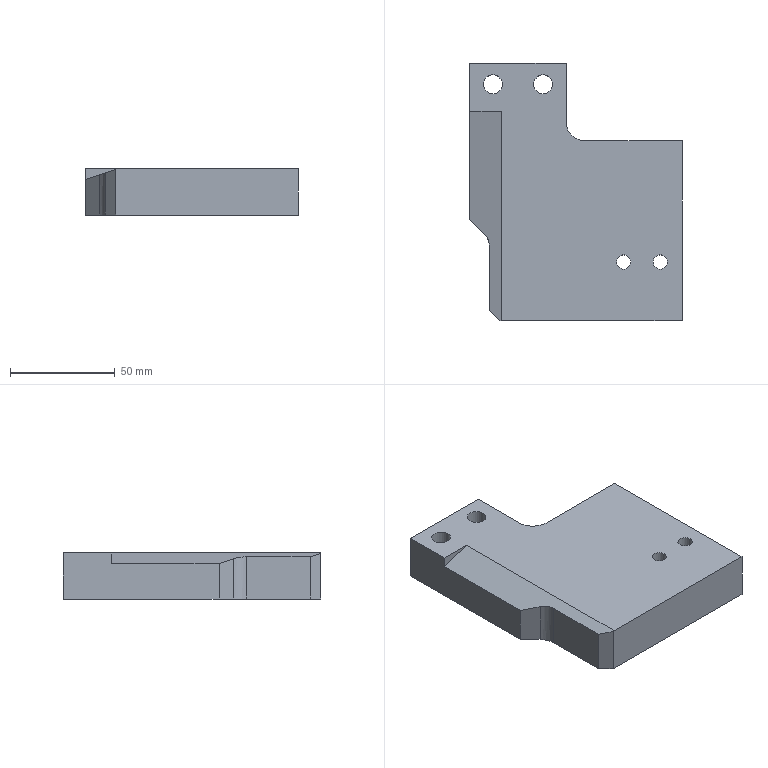Part | STEP file | gslz 2016.10.28-13_id782_x_t | 1 solid | 29 faces | box 101.5 x 123 x 22 mm | volume 209247 mm3 | plane 19 | cylinder 10 | commonest cylinder face diameters 9 x3 6.8 x2 14 x2 18 x2 6 x1